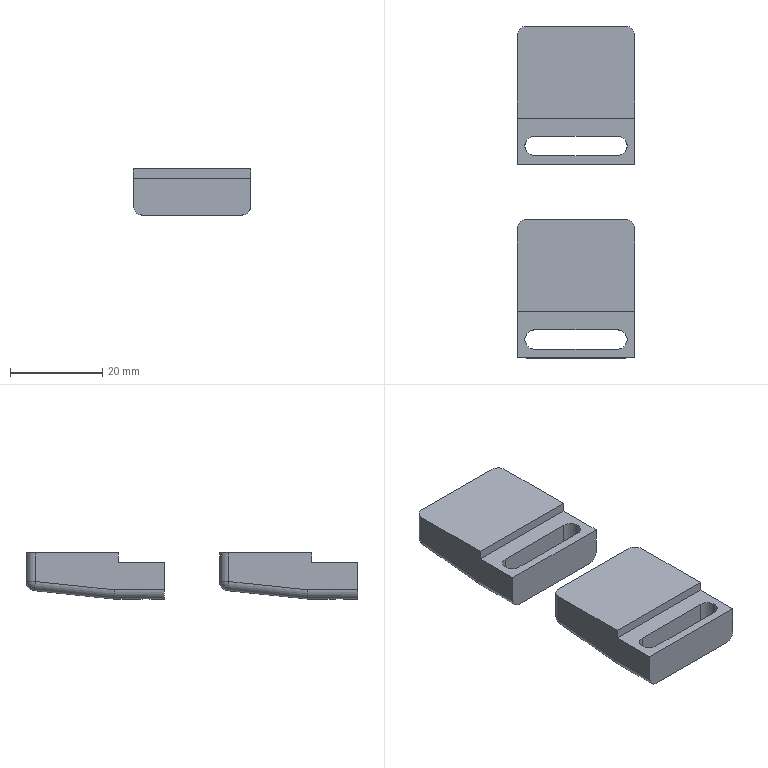NC program | NX | posted with a generic post | part box 25.5 x 72 x 10 mm
Whole program:
N10 G17 G21 G94 G90
(FLOOR_WALL_COPY , TOOL : D80)
N12 T19 M6
N14 G54
N16 G17 G0 G90 X83. Y0. B0. C0. S6500 M3
N18 G43 Z30. H19
N20 Z3.
N22 G94 G1 Z0. F1500.
N24 X78.
N26 X-78.
N28 X-83.
N30 Z3.
N32 G0 Z30.
N34 M5
(ZLEVEL_PROFILE , TOOL : D10)
N36 T15 M6
N38 G54
N40 G17 G0 G90 X-12.133 Y17.85 B0. C0. S9500 M3
N42 G43 Z30. H15
N44 Z1.5
N46 G94 G1 X-5.446 Z1.15 F1000.
N48 X-4.102 Y17.516 Z1.077
N50 X-2.896 Y16.834 Z1.004
N52 X-1.916 Y15.854 Z0.932
N54 X-1.234 Y14.648 Z0.859
N56 X-0.9 Y13.304 Z0.787
N58 Y-13.304 Z-0.608
N60 X-1.234 Y-14.648 Z-0.681
N62 X-1.916 Y-15.854 Z-0.753
N64 X-2.896 Y-16.834 Z-0.826
N66 X-4.102 Y-17.516 Z-0.898
N68 X-5.446 Y-17.85 Z-0.971
N70 X-6. Z-1.
N72 X-34. F3000.
N74 G2 X-41.1 Y-10.75 R7.1
N76 G1 Y10.75
N78 G2 X-34. Y17.85 R7.1
N80 G1 X-6.
N82 G2 X-0.9 Y12.75 R5.1
N84 G1 Y-12.75
N86 G2 X-6. Y-17.85 R5.1
N88 G1 X-33.871 Z-1.486
N90 X-34.258 Y-17.845 Z-1.493
N92 X-34.644 Y-17.821 Z-1.5
N94 X-35.028 Y-17.775 Z-1.507
N96 X-35.41 Y-17.709 Z-1.514
N98 X-35.787 Y-17.621 Z-1.52
N100 X-36.159 Y-17.514 Z-1.527
N102 X-36.524 Y-17.386 Z-1.534
N104 X-36.882 Y-17.239 Z-1.541
N106 X-37.231 Y-17.072 Z-1.547
N108 X-37.571 Y-16.887 Z-1.554
N110 X-37.9 Y-16.683 Z-1.561
N112 X-38.218 Y-16.462 Z-1.568
N114 X-38.523 Y-16.223 Z-1.574
N116 X-38.814 Y-15.969 Z-1.581
N118 X-39.091 Y-15.699 Z-1.588
N120 X-39.353 Y-15.414 Z-1.595
N122 X-39.6 Y-15.115 Z-1.601
N124 X-39.829 Y-14.804 Z-1.608
N126 X-40.041 Y-14.48 Z-1.615
N128 X-40.236 Y-14.145 Z-1.622
N130 X-40.411 Y-13.8 Z-1.628
N132 X-40.568 Y-13.446 Z-1.635
N134 X-40.705 Y-13.084 Z-1.642
N136 X-40.822 Y-12.716 Z-1.649
N138 X-40.919 Y-12.341 Z-1.655
N140 X-40.996 Y-11.961 Z-1.662
N142 X-41.052 Y-11.578 Z-1.669
N144 X-41.086 Y-11.193 Z-1.676
N146 X-41.1 Y-10.806 Z-1.682
N148 Y-10.419 Z-1.689
N150 Y7.387 Z-2.
N152 Y10.75
N154 G2 X-34. Y17.85 R7.1
N156 G1 X-6.
N158 G2 X-0.9 Y12.75 R5.1
N160 G1 Y-12.75
N162 G2 X-6. Y-17.85 R5.1
N164 G1 X-33.871 Z-2.486
N166 X-34.258 Y-17.845 Z-2.493
N168 X-34.644 Y-17.821 Z-2.5
N170 X-35.028 Y-17.775 Z-2.507
N172 X-35.41 Y-17.709 Z-2.514
N174 X-35.787 Y-17.621 Z-2.52
N176 X-36.159 Y-17.514 Z-2.527
N178 X-36.524 Y-17.386 Z-2.534
N180 X-36.882 Y-17.239 Z-2.541
N182 X-37.231 Y-17.072 Z-2.547
N184 X-37.571 Y-16.887 Z-2.554
N186 X-37.9 Y-16.683 Z-2.561
N188 X-38.218 Y-16.462 Z-2.568
N190 X-38.523 Y-16.223 Z-2.574
N192 X-38.814 Y-15.969 Z-2.581
N194 X-39.091 Y-15.699 Z-2.588
N196 X-39.353 Y-15.414 Z-2.595
N198 X-39.6 Y-15.115 Z-2.601
N200 X-39.829 Y-14.804 Z-2.608
N202 X-40.041 Y-14.48 Z-2.615
N204 X-40.236 Y-14.145 Z-2.622
N206 X-40.411 Y-13.8 Z-2.628
N208 X-40.568 Y-13.446 Z-2.635
N210 X-40.705 Y-13.084 Z-2.642
N212 X-40.822 Y-12.716 Z-2.649
N214 X-40.919 Y-12.341 Z-2.655
N216 X-40.996 Y-11.961 Z-2.662
N218 X-41.052 Y-11.578 Z-2.669
N220 X-41.086 Y-11.193 Z-2.676
N222 X-41.1 Y-10.806 Z-2.682
N224 Y-10.419 Z-2.689
N226 Y7.387 Z-3.
N228 Y10.75
N230 G2 X-34. Y17.85 R7.1
N232 G1 X-6.
N234 G2 X-0.9 Y12.75 R5.1
N236 G1 Y-12.75
N238 G2 X-6. Y-17.85 R5.1
N240 G1 X-33.871 Z-3.486
N242 X-34.258 Y-17.845 Z-3.493
N244 X-34.644 Y-17.821 Z-3.5
N246 X-35.028 Y-17.775 Z-3.507
N248 X-35.41 Y-17.709 Z-3.514
N250 X-35.787 Y-17.621 Z-3.52
N252 X-36.159 Y-17.514 Z-3.527
N254 X-36.524 Y-17.386 Z-3.534
N256 X-36.882 Y-17.239 Z-3.541
N258 X-37.231 Y-17.072 Z-3.547
N260 X-37.571 Y-16.887 Z-3.554
N262 X-37.9 Y-16.683 Z-3.561
N264 X-38.218 Y-16.462 Z-3.568
N266 X-38.523 Y-16.223 Z-3.574
N268 X-38.814 Y-15.969 Z-3.581
N270 X-39.091 Y-15.699 Z-3.588
N272 X-39.353 Y-15.414 Z-3.595
N274 X-39.6 Y-15.115 Z-3.601
N276 X-39.829 Y-14.804 Z-3.608
N278 X-40.041 Y-14.48 Z-3.615
N280 X-40.236 Y-14.145 Z-3.622
N282 X-40.411 Y-13.8 Z-3.628
N284 X-40.568 Y-13.446 Z-3.635
N286 X-40.705 Y-13.084 Z-3.642
N288 X-40.822 Y-12.716 Z-3.649
N290 X-40.919 Y-12.341 Z-3.655
N292 X-40.996 Y-11.961 Z-3.662
N294 X-41.052 Y-11.578 Z-3.669
N296 X-41.086 Y-11.193 Z-3.676
N298 X-41.1 Y-10.806 Z-3.682
N300 Y-10.419 Z-3.689
N302 Y7.387 Z-4.
N304 Y10.75
N306 G2 X-34. Y17.85 R7.1
N308 G1 X-6.
N310 G2 X-0.9 Y12.75 R5.1
N312 G1 Y-12.75
N314 G2 X-6. Y-17.85 R5.1
N316 G1 X-33.871 Z-4.486
N318 X-34.258 Y-17.845 Z-4.493
N320 X-34.644 Y-17.821 Z-4.5
N322 X-35.028 Y-17.775 Z-4.507
N324 X-35.41 Y-17.709 Z-4.514
N326 X-35.787 Y-17.621 Z-4.52
N328 X-36.159 Y-17.514 Z-4.527
N330 X-36.524 Y-17.386 Z-4.534
N332 X-36.882 Y-17.239 Z-4.541
N334 X-37.231 Y-17.072 Z-4.547
N336 X-37.571 Y-16.887 Z-4.554
N338 X-37.9 Y-16.683 Z-4.561
N340 X-38.218 Y-16.462 Z-4.568
N342 X-38.523 Y-16.223 Z-4.574
N344 X-38.814 Y-15.969 Z-4.581
N346 X-39.091 Y-15.699 Z-4.588
N348 X-39.353 Y-15.414 Z-4.595
N350 X-39.6 Y-15.115 Z-4.601
N352 X-39.829 Y-14.804 Z-4.608
N354 X-40.041 Y-14.48 Z-4.615
N356 X-40.236 Y-14.145 Z-4.622
N358 X-40.411 Y-13.8 Z-4.628
N360 X-40.568 Y-13.446 Z-4.635
N362 X-40.705 Y-13.084 Z-4.642
N364 X-40.822 Y-12.716 Z-4.649
N366 X-40.919 Y-12.341 Z-4.655
N368 X-40.996 Y-11.961 Z-4.662
N370 X-41.052 Y-11.578 Z-4.669
N372 X-41.086 Y-11.193 Z-4.676
N374 X-41.1 Y-10.806 Z-4.682
N376 Y-10.419 Z-4.689
N378 Y7.387 Z-5.
N380 Y10.75
N382 G2 X-34. Y17.85 R7.1
N384 G1 X-6.
N386 G2 X-0.9 Y12.75 R5.1
N388 G1 Y-12.75
N390 G2 X-6. Y-17.85 R5.1
N392 G1 X-33.871 Z-5.486
N394 X-34.258 Y-17.845 Z-5.493
N396 X-34.644 Y-17.821 Z-5.5
N398 X-35.028 Y-17.775 Z-5.507
N400 X-35.41 Y-17.709 Z-5.514
N402 X-35.787 Y-17.621 Z-5.52
N404 X-36.159 Y-17.514 Z-5.527
N406 X-36.524 Y-17.386 Z-5.534
N408 X-36.882 Y-17.239 Z-5.541
N410 X-37.231 Y-17.072 Z-5.547
N412 X-37.571 Y-16.887 Z-5.554
N414 X-37.9 Y-16.683 Z-5.561
N416 X-38.218 Y-16.462 Z-5.568
N418 X-38.523 Y-16.223 Z-5.574
N420 X-38.814 Y-15.969 Z-5.581
N422 X-39.091 Y-15.699 Z-5.588
N424 X-39.353 Y-15.414 Z-5.595
N426 X-39.6 Y-15.115 Z-5.601
N428 X-39.829 Y-14.804 Z-5.608
N430 X-40.041 Y-14.48 Z-5.615
N432 X-40.236 Y-14.145 Z-5.622
N434 X-40.411 Y-13.8 Z-5.628
N436 X-40.568 Y-13.446 Z-5.635
N438 X-40.705 Y-13.084 Z-5.642
N440 X-40.822 Y-12.716 Z-5.649
N442 X-40.919 Y-12.341 Z-5.655
N444 X-40.996 Y-11.961 Z-5.662
N446 X-41.052 Y-11.578 Z-5.669
N448 X-41.086 Y-11.193 Z-5.676
N450 X-41.1 Y-10.806 Z-5.682
N452 Y-10.419 Z-5.689
N454 Y7.387 Z-6.
N456 Y10.75
N458 G2 X-34. Y17.85 R7.1
N460 G1 X-6.
N462 G2 X-0.9 Y12.75 R5.1
N464 G1 Y-12.75
N466 G2 X-6. Y-17.85 R5.1
N468 G1 X-33.871 Z-6.486
N470 X-34.258 Y-17.845 Z-6.493
N472 X-34.644 Y-17.821 Z-6.5
N474 X-35.028 Y-17.775 Z-6.507
N476 X-35.41 Y-17.709 Z-6.514
N478 X-35.787 Y-17.621 Z-6.52
N480 X-36.159 Y-17.514 Z-6.527
N482 X-36.524 Y-17.386 Z-6.534
N484 X-36.882 Y-17.239 Z-6.541
N486 X-37.231 Y-17.072 Z-6.547
N488 X-37.571 Y-16.887 Z-6.554
N490 X-37.9 Y-16.683 Z-6.561
N492 X-38.218 Y-16.462 Z-6.568
N494 X-38.523 Y-16.223 Z-6.574
N496 X-38.814 Y-15.969 Z-6.581
N498 X-39.091 Y-15.699 Z-6.588
N500 X-39.353 Y-15.414 Z-6.595
N502 X-39.6 Y-15.115 Z-6.601
N504 X-39.829 Y-14.804 Z-6.608
N506 X-40.041 Y-14.48 Z-6.615
N508 X-40.236 Y-14.145 Z-6.622
N510 X-40.411 Y-13.8 Z-6.628
N512 X-40.568 Y-13.446 Z-6.635
N514 X-40.705 Y-13.084 Z-6.642
N516 X-40.822 Y-12.716 Z-6.649
N518 X-40.919 Y-12.341 Z-6.655
N520 X-40.996 Y-11.961 Z-6.662
N522 X-41.052 Y-11.578 Z-6.669
N524 X-41.086 Y-11.193 Z-6.676
N526 X-41.1 Y-10.806 Z-6.682
N528 Y-10.419 Z-6.689
N530 Y7.387 Z-7.
N532 Y10.75
N534 G2 X-34. Y17.85 R7.1
N536 G1 X-6.
N538 G2 X-0.9 Y12.75 R5.1
N540 G1 Y-12.75
N542 G2 X-6. Y-17.85 R5.1
N544 G1 X-33.871 Z-7.486
N546 X-34.258 Y-17.845 Z-7.493
N548 X-34.644 Y-17.821 Z-7.5
N550 X-35.028 Y-17.775 Z-7.507
N552 X-35.41 Y-17.709 Z-7.514
N554 X-35.787 Y-17.621 Z-7.52
N556 X-36.159 Y-17.514 Z-7.527
N558 X-36.524 Y-17.386 Z-7.534
N560 X-36.882 Y-17.239 Z-7.541
N562 X-37.231 Y-17.072 Z-7.547
N564 X-37.571 Y-16.887 Z-7.554
N566 X-37.9 Y-16.683 Z-7.561
N568 X-38.218 Y-16.462 Z-7.568
N570 X-38.523 Y-16.223 Z-7.574
N572 X-38.814 Y-15.969 Z-7.581
N574 X-39.091 Y-15.699 Z-7.588
N576 X-39.353 Y-15.414 Z-7.595
N578 X-39.6 Y-15.115 Z-7.601
N580 X-39.829 Y-14.804 Z-7.608
N582 X-40.041 Y-14.48 Z-7.615
N584 X-40.236 Y-14.145 Z-7.622
N586 X-40.411 Y-13.8 Z-7.628
N588 X-40.568 Y-13.446 Z-7.635
N590 X-40.705 Y-13.084 Z-7.642
N592 X-40.822 Y-12.716 Z-7.649
N594 X-40.919 Y-12.341 Z-7.655
N596 X-40.996 Y-11.961 Z-7.662
N598 X-41.052 Y-11.578 Z-7.669
N600 X-41.086 Y-11.193 Z-7.676
N602 X-41.1 Y-10.806 Z-7.682
N604 Y-10.419 Z-7.689
N606 Y7.387 Z-8.
N608 Y10.75
N610 G2 X-34. Y17.85 R7.1
N612 G1 X-6.
N614 G2 X-0.9 Y12.75 R5.1
N616 G1 Y-12.75
N618 G2 X-6. Y-17.85 R5.1
N620 G1 X-33.871 Z-8.486
N622 X-34.258 Y-17.845 Z-8.493
N624 X-34.644 Y-17.821 Z-8.5
N626 X-35.028 Y-17.775 Z-8.507
N628 X-35.41 Y-17.709 Z-8.514
N630 X-35.787 Y-17.621 Z-8.52
N632 X-36.159 Y-17.514 Z-8.527
N634 X-36.524 Y-17.386 Z-8.534
N636 X-36.882 Y-17.239 Z-8.541
N638 X-37.231 Y-17.072 Z-8.547
N640 X-37.571 Y-16.887 Z-8.554
N642 X-37.9 Y-16.683 Z-8.561
N644 X-38.218 Y-16.462 Z-8.568
N646 X-38.523 Y-16.223 Z-8.574
N648 X-38.814 Y-15.969 Z-8.581
N650 X-39.091 Y-15.699 Z-8.588
N652 X-39.353 Y-15.414 Z-8.595
N654 X-39.6 Y-15.115 Z-8.601
N656 X-39.829 Y-14.804 Z-8.608
N658 X-40.041 Y-14.48 Z-8.615
N660 X-40.236 Y-14.145 Z-8.622
N662 X-40.411 Y-13.8 Z-8.628
N664 X-40.568 Y-13.446 Z-8.635
N666 X-40.705 Y-13.084 Z-8.642
N668 X-40.822 Y-12.716 Z-8.649
N670 X-40.919 Y-12.341 Z-8.655
N672 X-40.996 Y-11.961 Z-8.662
N674 X-41.052 Y-11.578 Z-8.669
N676 X-41.086 Y-11.193 Z-8.676
N678 X-41.1 Y-10.806 Z-8.682
N680 Y-10.419 Z-8.689
N682 Y7.387 Z-9.
N684 Y10.75
N686 G2 X-34. Y17.85 R7.1
N688 G1 X-6.
N690 G2 X-0.9 Y12.75 R5.1
N692 G1 Y-12.75
N694 G2 X-6. Y-17.85 R5.1
N696 G1 X-33.871 Z-9.486
N698 X-34.258 Y-17.845 Z-9.493
N700 X-34.644 Y-17.821 Z-9.5
N702 X-35.028 Y-17.775 Z-9.507
N704 X-35.41 Y-17.709 Z-9.514
N706 X-35.787 Y-17.621 Z-9.52
N708 X-36.159 Y-17.514 Z-9.527
N710 X-36.524 Y-17.386 Z-9.534
N712 X-36.882 Y-17.239 Z-9.541
N714 X-37.231 Y-17.072 Z-9.547
N716 X-37.571 Y-16.887 Z-9.554
N718 X-37.9 Y-16.683 Z-9.561
N720 X-38.218 Y-16.462 Z-9.568
N722 X-38.523 Y-16.223 Z-9.574
N724 X-38.814 Y-15.969 Z-9.581
N726 X-39.091 Y-15.699 Z-9.588
N728 X-39.353 Y-15.414 Z-9.595
N730 X-39.6 Y-15.115 Z-9.601
N732 X-39.829 Y-14.804 Z-9.608
N734 X-40.041 Y-14.48 Z-9.615
N736 X-40.236 Y-14.145 Z-9.622
N738 X-40.411 Y-13.8 Z-9.628
N740 X-40.568 Y-13.446 Z-9.635
N742 X-40.705 Y-13.084 Z-9.642
N744 X-40.822 Y-12.716 Z-9.649
N746 X-40.919 Y-12.341 Z-9.655
N748 X-40.996 Y-11.961 Z-9.662
N750 X-41.052 Y-11.578 Z-9.669
N752 X-41.086 Y-11.193 Z-9.676
N754 X-41.1 Y-10.806 Z-9.682
N756 Y-10.419 Z-9.689
N758 Y7.387 Z-10.
N760 Y10.75
N762 G2 X-34. Y17.85 R7.1
N764 G1 X-6.
N766 G2 X-0.9 Y12.75 R5.1
N768 G1 Y-12.75
N770 G2 X-6. Y-17.85 R5.1
N772 G1 X-34.
N774 G2 X-41.1 Y-10.75 R7.1
N776 G1 Y7.387
N778 Z-8.5
N780 G0 Z53.
N782 X29.867 Y17.85
N784 Z1.5
N786 G1 X36.554 Z1.15 F1000.
N788 X37.898 Y17.516 Z1.077
N790 X39.104 Y16.834 Z1.004
N792 X40.084 Y15.854 Z0.932
N794 X40.766 Y14.648 Z0.859
N796 X41.1 Y13.304 Z0.787
N798 Y-13.304 Z-0.608
N800 X40.766 Y-14.648 Z-0.681
N802 X40.084 Y-15.854 Z-0.753
N804 X39.104 Y-16.834 Z-0.826
N806 X37.898 Y-17.516 Z-0.898
N808 X36.554 Y-17.85 Z-0.971
N810 X36. Z-1.
N812 X8. F3000.
N814 G2 X0.9 Y-10.75 R7.1
N816 G1 Y10.75
N818 G2 X8. Y17.85 R7.1
N820 G1 X36.
N822 G2 X41.1 Y12.75 R5.1
N824 G1 Y-12.75
N826 G2 X36. Y-17.85 R5.1
N828 G1 X8.129 Z-1.486
N830 X7.742 Y-17.845 Z-1.493
N832 X7.356 Y-17.821 Z-1.5
N834 X6.972 Y-17.775 Z-1.507
N836 X6.59 Y-17.709 Z-1.514
N838 X6.213 Y-17.621 Z-1.52
N840 X5.841 Y-17.514 Z-1.527
N842 X5.476 Y-17.386 Z-1.534
N844 X5.118 Y-17.239 Z-1.541
N846 X4.769 Y-17.072 Z-1.547
N848 X4.429 Y-16.887 Z-1.554
N850 X4.1 Y-16.683 Z-1.561
N852 X3.782 Y-16.462 Z-1.568
N854 X3.477 Y-16.223 Z-1.574
N856 X3.186 Y-15.969 Z-1.581
N858 X2.909 Y-15.699 Z-1.588
N860 X2.647 Y-15.414 Z-1.595
N862 X2.4 Y-15.115 Z-1.601
N864 X2.171 Y-14.804 Z-1.608
N866 X1.959 Y-14.48 Z-1.615
N868 X1.764 Y-14.145 Z-1.622
N870 X1.589 Y-13.8 Z-1.628
N872 X1.432 Y-13.446 Z-1.635
N874 X1.295 Y-13.084 Z-1.642
N876 X1.178 Y-12.716 Z-1.649
N878 X1.081 Y-12.341 Z-1.655
N880 X1.004 Y-11.961 Z-1.662
N882 X0.948 Y-11.578 Z-1.669
N884 X0.914 Y-11.193 Z-1.676
N886 X0.9 Y-10.806 Z-1.682
N888 Y-10.419 Z-1.689
N890 Y7.387 Z-2.
N892 Y10.75
N894 G2 X8. Y17.85 R7.1
N896 G1 X36.
N898 G2 X41.1 Y12.75 R5.1
N900 G1 Y-12.75
N902 G2 X36. Y-17.85 R5.1
N904 G1 X8.129 Z-2.486
N906 X7.742 Y-17.845 Z-2.493
N908 X7.356 Y-17.821 Z-2.5
N910 X6.972 Y-17.775 Z-2.507
N912 X6.59 Y-17.709 Z-2.514
N914 X6.213 Y-17.621 Z-2.52
N916 X5.841 Y-17.514 Z-2.527
N918 X5.476 Y-17.386 Z-2.534
N920 X5.118 Y-17.239 Z-2.541
N922 X4.769 Y-17.072 Z-2.547
N924 X4.429 Y-16.887 Z-2.554
N926 X4.1 Y-16.683 Z-2.561
N928 X3.782 Y-16.462 Z-2.568
N930 X3.477 Y-16.223 Z-2.574
N932 X3.186 Y-15.969 Z-2.581
N934 X2.909 Y-15.699 Z-2.588
N936 X2.647 Y-15.414 Z-2.595
N938 X2.4 Y-15.115 Z-2.601
N940 X2.171 Y-14.804 Z-2.608
N942 X1.959 Y-14.48 Z-2.615
N944 X1.764 Y-14.145 Z-2.622
N946 X1.589 Y-13.8 Z-2.628
N948 X1.432 Y-13.446 Z-2.635
N950 X1.295 Y-13.084 Z-2.642
N952 X1.178 Y-12.716 Z-2.649
N954 X1.081 Y-12.341 Z-2.655
N956 X1.004 Y-11.961 Z-2.662
N958 X0.948 Y-11.578 Z-2.669
N960 X0.914 Y-11.193 Z-2.676
N962 X0.9 Y-10.806 Z-2.682
N964 Y-10.419 Z-2.689
N966 Y7.387 Z-3.
N968 Y10.75
N970 G2 X8. Y17.85 R7.1
N972 G1 X36.
N974 G2 X41.1 Y12.75 R5.1
N976 G1 Y-12.75
N978 G2 X36. Y-17.85 R5.1
N980 G1 X8.129 Z-3.486
N982 X7.742 Y-17.845 Z-3.493
N984 X7.356 Y-17.821 Z-3.5
N986 X6.972 Y-17.775 Z-3.507
N988 X6.59 Y-17.709 Z-3.514
N990 X6.213 Y-17.621 Z-3.52
N992 X5.841 Y-17.514 Z-3.527
N994 X5.476 Y-17.386 Z-3.534
N996 X5.118 Y-17.239 Z-3.541
N998 X4.769 Y-17.072 Z-3.547
N1000 X4.429 Y-16.887 Z-3.554
N1002 X4.1 Y-16.683 Z-3.561
N1004 X3.782 Y-16.462 Z-3.568
N1006 X3.477 Y-16.223 Z-3.574
N1008 X3.186 Y-15.969 Z-3.581
N1010 X2.909 Y-15.699 Z-3.588
N1012 X2.647 Y-15.414 Z-3.595
N1014 X2.4 Y-15.115 Z-3.601
N1016 X2.171 Y-14.804 Z-3.608
N1018 X1.959 Y-14.48 Z-3.615
N1020 X1.764 Y-14.145 Z-3.622
N1022 X1.589 Y-13.8 Z-3.628
N1024 X1.432 Y-13.446 Z-3.635
N1026 X1.295 Y-13.084 Z-3.642
N1028 X1.178 Y-12.716 Z-3.649
N1030 X1.081 Y-12.341 Z-3.655
N1032 X1.004 Y-11.961 Z-3.662
N1034 X0.948 Y-11.578 Z-3.669
N1036 X0.914 Y-11.193 Z-3.676
N1038 X0.9 Y-10.806 Z-3.682
N1040 Y-10.419 Z-3.689
N1042 Y7.387 Z-4.
N1044 Y10.75
N1046 G2 X8. Y17.85 R7.1
N1048 G1 X36.
N1050 G2 X41.1 Y12.75 R5.1
N1052 G1 Y-12.75
N1054 G2 X36. Y-17.85 R5.1
N1056 G1 X8.129 Z-4.486
N1058 X7.742 Y-17.845 Z-4.493
N1060 X7.356 Y-17.821 Z-4.5
N1062 X6.972 Y-17.775 Z-4.507
N1064 X6.59 Y-17.709 Z-4.514
N1066 X6.213 Y-17.621 Z-4.52
N1068 X5.841 Y-17.514 Z-4.527
N1070 X5.476 Y-17.386 Z-4.534
N1072 X5.118 Y-17.239 Z-4.541
N1074 X4.769 Y-17.072 Z-4.547
N1076 X4.429 Y-16.887 Z-4.554
N1078 X4.1 Y-16.683 Z-4.561
N1080 X3.782 Y-16.462 Z-4.568
N1082 X3.477 Y-16.223 Z-4.574
N1084 X3.186 Y-15.969 Z-4.581
N1086 X2.909 Y-15.699 Z-4.588
N1088 X2.647 Y-15.414 Z-4.595
N1090 X2.4 Y-15.115 Z-4.601
N1092 X2.171 Y-14.804 Z-4.608
N1094 X1.959 Y-14.48 Z-4.615
N1096 X1.764 Y-14.145 Z-4.622
N1098 X1.589 Y-13.8 Z-4.628
N1100 X1.432 Y-13.446 Z-4.635
N1102 X1.295 Y-13.084 Z-4.642
N1104 X1.178 Y-12.716 Z-4.649
N1106 X1.081 Y-12.341 Z-4.655
N1108 X1.004 Y-11.961 Z-4.662
N1110 X0.948 Y-11.578 Z-4.669
N1112 X0.914 Y-11.193 Z-4.676
N1114 X0.9 Y-10.806 Z-4.682
N1116 Y-10.419 Z-4.689
N1118 Y7.387 Z-5.
N1120 Y10.75
N1122 G2 X8. Y17.85 R7.1
N1124 G1 X36.
N1126 G2 X41.1 Y12.75 R5.1
N1128 G1 Y-12.75
N1130 G2 X36. Y-17.85 R5.1
N1132 G1 X8.129 Z-5.486
N1134 X7.742 Y-17.845 Z-5.493
N1136 X7.356 Y-17.821 Z-5.5
N1138 X6.972 Y-17.775 Z-5.507
N1140 X6.59 Y-17.709 Z-5.514
N1142 X6.213 Y-17.621 Z-5.52
N1144 X5.841 Y-17.514 Z-5.527
N1146 X5.476 Y-17.386 Z-5.534
N1148 X5.118 Y-17.239 Z-5.541
N1150 X4.769 Y-17.072 Z-5.547
N1152 X4.429 Y-16.887 Z-5.554
N1154 X4.1 Y-16.683 Z-5.561
N1156 X3.782 Y-16.462 Z-5.568
N1158 X3.477 Y-16.223 Z-5.574
N1160 X3.186 Y-15.969 Z-5.581
N1162 X2.909 Y-15.699 Z-5.588
N1164 X2.647 Y-15.414 Z-5.595
N1166 X2.4 Y-15.115 Z-5.601
N1168 X2.171 Y-14.804 Z-5.608
N1170 X1.959 Y-14.48 Z-5.615
N1172 X1.764 Y-14.145 Z-5.622
N1174 X1.589 Y-13.8 Z-5.628
N1176 X1.432 Y-13.446 Z-5.635
N1178 X1.295 Y-13.084 Z-5.642
N1180 X1.178 Y-12.716 Z-5.649
N1182 X1.081 Y-12.341 Z-5.655
N1184 X1.004 Y-11.961 Z-5.662
N1186 X0.948 Y-11.578 Z-5.669
N1188 X0.914 Y-11.193 Z-5.676
N1190 X0.9 Y-10.806 Z-5.682
N1192 Y-10.419 Z-5.689
N1194 Y7.387 Z-6.
N1196 Y10.75
N1198 G2 X8. Y17.85 R7.1
N1200 G1 X36.
N1202 G2 X41.1 Y12.75 R5.1
N1204 G1 Y-12.75
N1206 G2 X36. Y-17.85 R5.1
N1208 G1 X8.129 Z-6.486
N1210 X7.742 Y-17.845 Z-6.493
N1212 X7.356 Y-17.821 Z-6.5
N1214 X6.972 Y-17.775 Z-6.507
N1216 X6.59 Y-17.709 Z-6.514
N1218 X6.213 Y-17.621 Z-6.52
N1220 X5.841 Y-17.514 Z-6.527
N1222 X5.476 Y-17.386 Z-6.534
N1224 X5.118 Y-17.239 Z-6.541
N1226 X4.769 Y-17.072 Z-6.547
N1228 X4.429 Y-16.887 Z-6.554
N1230 X4.1 Y-16.683 Z-6.561
N1232 X3.782 Y-16.462 Z-6.568
N1234 X3.477 Y-16.223 Z-6.574
N1236 X3.186 Y-15.969 Z-6.581
N1238 X2.909 Y-15.699 Z-6.588
N1240 X2.647 Y-15.414 Z-6.595
N1242 X2.4 Y-15.115 Z-6.601
N1244 X2.171 Y-14.804 Z-6.608
N1246 X1.959 Y-14.48 Z-6.615
N1248 X1.764 Y-14.145 Z-6.622
N1250 X1.589 Y-13.8 Z-6.628
N1252 X1.432 Y-13.446 Z-6.635
N1254 X1.295 Y-13.084 Z-6.642
N1256 X1.178 Y-12.716 Z-6.649
N1258 X1.081 Y-12.341 Z-6.655
N1260 X1.004 Y-11.961 Z-6.662
N1262 X0.948 Y-11.578 Z-6.669
N1264 X0.914 Y-11.193 Z-6.676
N1266 X0.9 Y-10.806 Z-6.682
N1268 Y-10.419 Z-6.689
N1270 Y7.387 Z-7.
N1272 Y10.75
N1274 G2 X8. Y17.85 R7.1
N1276 G1 X36.
N1278 G2 X41.1 Y12.75 R5.1
N1280 G1 Y-12.75
N1282 G2 X36. Y-17.85 R5.1
N1284 G1 X8.129 Z-7.486
N1286 X7.742 Y-17.845 Z-7.493
N1288 X7.356 Y-17.821 Z-7.5
N1290 X6.972 Y-17.775 Z-7.507
N1292 X6.59 Y-17.709 Z-7.514
N1294 X6.213 Y-17.621 Z-7.52
N1296 X5.841 Y-17.514 Z-7.527
N1298 X5.476 Y-17.386 Z-7.534
N1300 X5.118 Y-17.239 Z-7.541
N1302 X4.769 Y-17.072 Z-7.547
N1304 X4.429 Y-16.887 Z-7.554
N1306 X4.1 Y-16.683 Z-7.561
N1308 X3.782 Y-16.462 Z-7.568
N1310 X3.477 Y-16.223 Z-7.574
N1312 X3.186 Y-15.969 Z-7.581
N1314 X2.909 Y-15.699 Z-7.588
N1316 X2.647 Y-15.414 Z-7.595
N1318 X2.4 Y-15.115 Z-7.601
N1320 X2.171 Y-14.804 Z-7.608
N1322 X1.959 Y-14.48 Z-7.615
N1324 X1.764 Y-14.145 Z-7.622
N1326 X1.589 Y-13.8 Z-7.628
N1328 X1.432 Y-13.446 Z-7.635
N1330 X1.295 Y-13.084 Z-7.642
N1332 X1.178 Y-12.716 Z-7.649
N1334 X1.081 Y-12.341 Z-7.655
N1336 X1.004 Y-11.961 Z-7.662
N1338 X0.948 Y-11.578 Z-7.669
N1340 X0.914 Y-11.193 Z-7.676
N1342 X0.9 Y-10.806 Z-7.682
N1344 Y-10.419 Z-7.689
N1346 Y7.387 Z-8.
N1348 Y10.75
N1350 G2 X8. Y17.85 R7.1
N1352 G1 X36.
N1354 G2 X41.1 Y12.75 R5.1
N1356 G1 Y-12.75
N1358 G2 X36. Y-17.85 R5.1
N1360 G1 X8.129 Z-8.486
N1362 X7.742 Y-17.845 Z-8.493
N1364 X7.356 Y-17.821 Z-8.5
N1366 X6.972 Y-17.775 Z-8.507
N1368 X6.59 Y-17.709 Z-8.514
N1370 X6.213 Y-17.621 Z-8.52
N1372 X5.841 Y-17.514 Z-8.527
N1374 X5.476 Y-17.386 Z-8.534
N1376 X5.118 Y-17.239 Z-8.541
N1378 X4.769 Y-17.072 Z-8.547
N1380 X4.429 Y-16.887 Z-8.554
N1382 X4.1 Y-16.683 Z-8.561
N1384 X3.782 Y-16.462 Z-8.568
N1386 X3.477 Y-16.223 Z-8.574
N1388 X3.186 Y-15.969 Z-8.581
N1390 X2.909 Y-15.699 Z-8.588
N1392 X2.647 Y-15.414 Z-8.595
N1394 X2.4 Y-15.115 Z-8.601
N1396 X2.171 Y-14.804 Z-8.608
N1398 X1.959 Y-14.48 Z-8.615
N1400 X1.764 Y-14.145 Z-8.622
N1402 X1.589 Y-13.8 Z-8.628
N1404 X1.432 Y-13.446 Z-8.635
N1406 X1.295 Y-13.084 Z-8.642
N1408 X1.178 Y-12.716 Z-8.649
N1410 X1.081 Y-12.341 Z-8.655
N1412 X1.004 Y-11.961 Z-8.662
N1414 X0.948 Y-11.578 Z-8.669
N1416 X0.914 Y-11.193 Z-8.676
N1418 X0.9 Y-10.806 Z-8.682
N1420 Y-10.419 Z-8.689
N1422 Y7.387 Z-9.
N1424 Y10.75
N1426 G2 X8. Y17.85 R7.1
N1428 G1 X36.
N1430 G2 X41.1 Y12.75 R5.1
N1432 G1 Y-12.75
N1434 G2 X36. Y-17.85 R5.1
N1436 G1 X8.129 Z-9.486
N1438 X7.742 Y-17.845 Z-9.493
N1440 X7.356 Y-17.821 Z-9.5
N1442 X6.972 Y-17.775 Z-9.507
N1444 X6.59 Y-17.709 Z-9.514
N1446 X6.213 Y-17.621 Z-9.52
N1448 X5.841 Y-17.514 Z-9.527
N1450 X5.476 Y-17.386 Z-9.534
N1452 X5.118 Y-17.239 Z-9.541
N1454 X4.769 Y-17.072 Z-9.547
N1456 X4.429 Y-16.887 Z-9.554
N1458 X4.1 Y-16.683 Z-9.561
N1460 X3.782 Y-16.462 Z-9.568
N1462 X3.477 Y-16.223 Z-9.574
N1464 X3.186 Y-15.969 Z-9.581
N1466 X2.909 Y-15.699 Z-9.588
N1468 X2.647 Y-15.414 Z-9.595
N1470 X2.4 Y-15.115 Z-9.601
N1472 X2.171 Y-14.804 Z-9.608
N1474 X1.959 Y-14.48 Z-9.615
N1476 X1.764 Y-14.145 Z-9.622
N1478 X1.589 Y-13.8 Z-9.628
N1480 X1.432 Y-13.446 Z-9.635
N1482 X1.295 Y-13.084 Z-9.642
N1484 X1.178 Y-12.716 Z-9.649
N1486 X1.081 Y-12.341 Z-9.655
N1488 X1.004 Y-11.961 Z-9.662
N1490 X0.948 Y-11.578 Z-9.669
N1492 X0.914 Y-11.193 Z-9.676
N1494 X0.9 Y-10.806 Z-9.682
N1496 Y-10.419 Z-9.689
N1498 Y7.387 Z-10.
N1500 Y10.75
N1502 G2 X8. Y17.85 R7.1
N1504 G1 X36.
N1506 G2 X41.1 Y12.75 R5.1
N1508 G1 Y-12.75
N1510 G2 X36. Y-17.85 R5.1
N1512 G1 X8.
N1514 G2 X0.9 Y-10.75 R7.1
N1516 G1 Y7.387
N1518 Z-8.5
N1520 G0 Z30.
(FLOOR_WALL , TOOL : D10)
N1522 X-7.393 Y19.25
N1524 Z0.05
N1526 G1 Z-0.95 F1000.
N1528 X-6.816 Y18.25
N1530 G3 X-5.95 Y17.75 R1.
N1532 G1 X-1. F2500.
N1534 Y-17.75
N1536 X-10.9
N1538 Y17.75
N1540 X-5.95
N1542 Y13.25
N1544 X-5.5
N1546 Y-13.25
N1548 X-6.4
N1550 Y13.25
N1552 X-5.95
N1554 G3 X-5.084 Y13.75 R1.
N1556 G1 Z0.05
N1558 G0 X-7.393 Y19.25 Z-0.9
N1560 G1 Z-1.9 F1000.
N1562 X-6.816 Y18.25
N1564 G3 X-5.95 Y17.75 R1.
N1566 G1 X-1. F2500.
N1568 Y-17.75
N1570 X-10.9
N1572 Y17.75
N1574 X-5.95
N1576 Y13.25
N1578 X-5.5
N1580 Y-13.25
N1582 X-6.4
N1584 Y13.25
N1586 X-5.95
N1588 G3 X-5.084 Y13.75 R1.
N1590 G1 Z-0.9
N1592 G0 Z30.
N1594 X42.5 Y1.443
N1596 Z0.05
N1598 G1 Z-0.95 F1000.
N1600 X41.5 Y0.866
N1602 G3 X41. Y0. R1.
N1604 G1 Y-17.75 F2500.
N1606 X31.1
N1608 Y17.75
N1610 X41.
N1612 Y0.
N1614 X36.5
N1616 Y-13.25
N1618 X35.6
N1620 Y13.25
N1622 X36.5
N1624 Y0.
N1626 G3 X37. Y-0.866 R1.
N1628 G1 Z0.05
N1630 G0 X42.5 Y1.443 Z-0.9
N1632 G1 Z-1.9 F1000.
N1634 X41.5 Y0.866
N1636 G3 X41. Y0. R1.
N1638 G1 Y-17.75 F2500.
N1640 X31.1
N1642 Y17.75
N1644 X41.
N1646 Y0.
N1648 X36.5
N1650 Y-13.25
N1652 X35.6
N1654 Y13.25
N1656 X36.5
N1658 Y0.
N1660 G3 X37. Y-0.866 R1.
N1662 G1 Z-0.9
N1664 G0 Z30.
N1666 M5
(ZLEVEL_PROFILE_COPY_1_COPY_COPY_1 , TOOL : D10JING)
N1668 T14 M6
N1670 G54
N1672 G17 G0 G90 X-4.378 Y-19.559 B0. C0. S9500 M3
N1674 G43 Z30. H14
N1676 Z-9.
N1678 G94 G1 Z-10. F1000.
N1680 X-5.134 Y-18.25
N1682 G3 X-6. Y-17.75 R1.
N1684 G1 X-34. F1200.
N1686 G2 X-41. Y-10.75 R7.
N1688 G1 Y10.75
N1690 G2 X-34. Y17.75 R7.
N1692 G1 X-6.
N1694 G2 X-1. Y12.75 R5.
N1696 G1 Y-12.75
N1698 G2 X-6. Y-17.75 R5.
N1700 G3 X-6.866 Y-18.25 R1.
N1702 G1 X-7.732 Y-19.75
N1704 Z-9.
N1706 G0 Z30.
N1708 X37.622 Y-19.559
N1710 Z-9.
N1712 G1 Z-10. F1000.
N1714 X36.866 Y-18.25
N1716 G3 X36. Y-17.75 R1.
N1718 G1 X8. F1200.
N1720 G2 X1. Y-10.75 R7.
N1722 G1 Y10.75
N1724 G2 X8. Y17.75 R7.
N1726 G1 X36.
N1728 G2 X41. Y12.75 R5.
N1730 G1 Y-12.75
N1732 G2 X36. Y-17.75 R5.
N1734 G3 X35.134 Y-18.25 R1.
N1736 G1 X34.268 Y-19.75
N1738 Z-9.
N1740 G0 Z30.
(FLOOR_WALL_1 , TOOL : D10JING)
N1742 X-5.5 Y-5.971
N1744 Z-0.4
N1746 G1 Y0. Z-2. F1250.
N1748 Y13.25
N1750 X-6.
N1752 Y-13.25
N1754 X-5.5
N1756 Y0.
N1758 X-1.
N1760 Y17.75
N1762 X-10.5
N1764 Y-17.75
N1766 X-1.
N1768 Y0.
N1770 G2 X-0.5 Y0.866 R1.
N1772 G1 Z-0.5
N1774 G0 Z30.
N1776 X-9.402 Y19.25
N1778 Z-0.5
N1780 G1 Z-2.
N1782 X-10.5 Y18.616
N1784 G3 X-11. Y17.75 R1.
N1786 G1 Y-17.75
N1788 G3 X-10.5 Y-18.616 R1.
N1790 G1 X-9.402 Y-19.25
N1792 Z-0.5
N1794 G0 Z30.
N1796 X36.5 Y-5.971
N1798 Z-0.4
N1800 G1 Y0. Z-2.
N1802 Y13.25
N1804 X36.
N1806 Y-13.25
N1808 X36.5
N1810 Y0.
N1812 X41.
N1814 Y17.75
N1816 X31.5
N1818 Y-17.75
N1820 X41.
N1822 Y0.
N1824 G2 X41.5 Y0.866 R1.
N1826 G1 X42.5 Y1.443
N1828 Z-0.5
N1830 G0 Z30.
N1832 X32.598 Y19.25
N1834 Z-0.5
N1836 G1 Z-2.
N1838 X31.5 Y18.616
N1840 G3 X31. Y17.75 R1.
N1842 G1 Y-17.75
N1844 G3 X31.5 Y-18.616 R1.
N1846 G1 X32.598 Y-19.25
N1848 Z-0.5
N1850 G0 Z30.
N1852 M5
(ZLEVEL_PROFILE_COPY , TOOL : D3)
N1854 T17 M6
N1856 G54
N1858 G17 G0 G90 X-9.4 Y-3.382 B0. C0. S9500 M3
N1860 G43 Z30. H17
N1862 Z-0.5
N1864 G94 G1 Y9.192 Z-1.159 F1000.
N1866 X-9.644 Y9.52 Z-1.18
N1868 X-10.038 Y9.629 Z-1.202
N1870 X-10.396 Y9.49 Z-1.222
N1872 X-10.6 Y9.192 Z-1.241
N1874 Y-9.192 Z-2.204
N1876 X-10.396 Y-9.49 Z-2.223
N1878 X-10.038 Y-9.629 Z-2.243
N1880 X-9.644 Y-9.52 Z-2.265
N1882 X-9.4 Y-9.192 Z-2.286
N1884 Y-9. Z-2.296
N1886 Y9. F1200.
N1888 G3 X-10. Y9.6 R0.6
N1890 X-10.6 Y9. R0.6
N1892 G1 Y-9.
N1894 G3 X-10. Y-9.6 R0.6
N1896 X-9.4 Y-9. R0.6
N1898 G1 Y7.975 Z-2.593
N1900 Y9.
N1902 G3 X-10. Y9.6 R0.6
N1904 X-10.6 Y9. R0.6
N1906 G1 Y-9.
N1908 G3 X-10. Y-9.6 R0.6
N1910 X-9.4 Y-9. R0.6
N1912 G1 Y7.975 Z-2.889
N1914 Y9.
N1916 G3 X-10. Y9.6 R0.6
N1918 X-10.6 Y9. R0.6
N1920 G1 Y-9.
N1922 G3 X-10. Y-9.6 R0.6
N1924 X-9.4 Y-9. R0.6
N1926 G1 Y7.975 Z-3.185
N1928 Y9.
N1930 G3 X-10. Y9.6 R0.6
N1932 X-10.6 Y9. R0.6
N1934 G1 Y-9.
N1936 G3 X-10. Y-9.6 R0.6
N1938 X-9.4 Y-9. R0.6
N1940 G1 Y7.975 Z-3.481
N1942 Y9.
N1944 G3 X-10. Y9.6 R0.6
N1946 X-10.6 Y9. R0.6
N1948 G1 Y-9.
N1950 G3 X-10. Y-9.6 R0.6
N1952 X-9.4 Y-9. R0.6
N1954 G1 Y7.975 Z-3.778
N1956 Y9.
N1958 G3 X-10. Y9.6 R0.6
N1960 X-10.6 Y9. R0.6
N1962 G1 Y-9.
N1964 G3 X-10. Y-9.6 R0.6
N1966 X-9.4 Y-9. R0.6
N1968 G1 Y7.975 Z-4.074
N1970 Y9.
N1972 G3 X-10. Y9.6 R0.6
N1974 X-10.6 Y9. R0.6
N1976 G1 Y-9.
N1978 G3 X-10. Y-9.6 R0.6
N1980 X-9.4 Y-9. R0.6
N1982 G1 Y7.975 Z-4.37
N1984 Y9.
N1986 G3 X-10. Y9.6 R0.6
N1988 X-10.6 Y9. R0.6
N1990 G1 Y-9.
N1992 G3 X-10. Y-9.6 R0.6
N1994 X-9.4 Y-9. R0.6
N1996 G1 Y7.975 Z-4.667
N1998 Y9.
N2000 G3 X-10. Y9.6 R0.6
N2002 X-10.6 Y9. R0.6
N2004 G1 Y-9.
N2006 G3 X-10. Y-9.6 R0.6
N2008 X-9.4 Y-9. R0.6
N2010 G1 Y7.975 Z-4.963
N2012 Y9.
N2014 G3 X-10. Y9.6 R0.6
N2016 X-10.6 Y9. R0.6
N2018 G1 Y-9.
N2020 G3 X-10. Y-9.6 R0.6
N2022 X-9.4 Y-9. R0.6
N2024 G1 Y7.975 Z-5.259
N2026 Y9.
N2028 G3 X-10. Y9.6 R0.6
N2030 X-10.6 Y9. R0.6
N2032 G1 Y-9.
N2034 G3 X-10. Y-9.6 R0.6
N2036 X-9.4 Y-9. R0.6
N2038 G1 Y7.975 Z-5.556
N2040 Y9.
N2042 G3 X-10. Y9.6 R0.6
N2044 X-10.6 Y9. R0.6
N2046 G1 Y-9.
N2048 G3 X-10. Y-9.6 R0.6
N2050 X-9.4 Y-9. R0.6
N2052 G1 Y7.975 Z-5.852
N2054 Y9.
N2056 G3 X-10. Y9.6 R0.6
N2058 X-10.6 Y9. R0.6
N2060 G1 Y-9.
N2062 G3 X-10. Y-9.6 R0.6
N2064 X-9.4 Y-9. R0.6
N2066 G1 Y7.975 Z-6.148
N2068 Y9.
N2070 G3 X-10. Y9.6 R0.6
N2072 X-10.6 Y9. R0.6
N2074 G1 Y-9.
N2076 G3 X-10. Y-9.6 R0.6
N2078 X-9.4 Y-9. R0.6
N2080 G1 Y7.975 Z-6.444
N2082 Y9.
N2084 G3 X-10. Y9.6 R0.6
N2086 X-10.6 Y9. R0.6
N2088 G1 Y-9.
N2090 G3 X-10. Y-9.6 R0.6
N2092 X-9.4 Y-9. R0.6
N2094 G1 Y7.975 Z-6.741
N2096 Y9.
N2098 G3 X-10. Y9.6 R0.6
N2100 X-10.6 Y9. R0.6
N2102 G1 Y-9.
N2104 G3 X-10. Y-9.6 R0.6
N2106 X-9.4 Y-9. R0.6
N2108 G1 Y7.975 Z-7.037
N2110 Y9.
N2112 G3 X-10. Y9.6 R0.6
N2114 X-10.6 Y9. R0.6
N2116 G1 Y-9.
N2118 G3 X-10. Y-9.6 R0.6
N2120 X-9.4 Y-9. R0.6
N2122 G1 Y7.975 Z-7.333
N2124 Y9.
N2126 G3 X-10. Y9.6 R0.6
N2128 X-10.6 Y9. R0.6
N2130 G1 Y-9.
N2132 G3 X-10. Y-9.6 R0.6
N2134 X-9.4 Y-9. R0.6
N2136 G1 Y7.975 Z-7.63
N2138 Y9.
N2140 G3 X-10. Y9.6 R0.6
N2142 X-10.6 Y9. R0.6
N2144 G1 Y-9.
N2146 G3 X-10. Y-9.6 R0.6
N2148 X-9.4 Y-9. R0.6
N2150 G1 Y7.975 Z-7.926
N2152 Y9.
N2154 G3 X-10. Y9.6 R0.6
N2156 X-10.6 Y9. R0.6
N2158 G1 Y-9.
N2160 G3 X-10. Y-9.6 R0.6
N2162 X-9.4 Y-9. R0.6
N2164 G1 Y7.975 Z-8.222
N2166 Y9.
N2168 G3 X-10. Y9.6 R0.6
N2170 X-10.6 Y9. R0.6
N2172 G1 Y-9.
N2174 G3 X-10. Y-9.6 R0.6
N2176 X-9.4 Y-9. R0.6
N2178 G1 Y7.975 Z-8.519
N2180 Y9.
N2182 G3 X-10. Y9.6 R0.6
N2184 X-10.6 Y9. R0.6
N2186 G1 Y-9.
N2188 G3 X-10. Y-9.6 R0.6
N2190 X-9.4 Y-9. R0.6
N2192 G1 Y7.975 Z-8.815
N2194 Y9.
N2196 G3 X-10. Y9.6 R0.6
N2198 X-10.6 Y9. R0.6
N2200 G1 Y-9.
N2202 G3 X-10. Y-9.6 R0.6
N2204 X-9.4 Y-9. R0.6
N2206 G1 Y7.975 Z-9.111
N2208 Y9.
N2210 G3 X-10. Y9.6 R0.6
N2212 X-10.6 Y9. R0.6
N2214 G1 Y-9.
N2216 G3 X-10. Y-9.6 R0.6
N2218 X-9.4 Y-9. R0.6
N2220 G1 Y7.975 Z-9.407
N2222 Y9.
N2224 G3 X-10. Y9.6 R0.6
N2226 X-10.6 Y9. R0.6
N2228 G1 Y-9.
N2230 G3 X-10. Y-9.6 R0.6
N2232 X-9.4 Y-9. R0.6
N2234 G1 Y7.975 Z-9.704
N2236 Y9.
N2238 G3 X-10. Y9.6 R0.6
N2240 X-10.6 Y9. R0.6
N2242 G1 Y-9.
N2244 G3 X-10. Y-9.6 R0.6
N2246 X-9.4 Y-9. R0.6
N2248 G1 Y7.975 Z-10.
N2250 Y9.
N2252 G3 X-10. Y9.6 R0.6
N2254 X-10.6 Y9. R0.6
N2256 G1 Y-9.
N2258 G3 X-10. Y-9.6 R0.6
N2260 X-9.4 Y-9. R0.6
N2262 G1 Y7.975
N2264 Z-8.5
N2266 G0 Z30.
N2268 X32.6 Y-3.382
N2270 Z-0.5
N2272 G1 Y9.192 Z-1.159 F1000.
N2274 X32.356 Y9.52 Z-1.18
N2276 X31.962 Y9.629 Z-1.202
N2278 X31.604 Y9.49 Z-1.222
N2280 X31.4 Y9.192 Z-1.241
N2282 Y-9.192 Z-2.204
N2284 X31.604 Y-9.49 Z-2.223
N2286 X31.962 Y-9.629 Z-2.243
N2288 X32.356 Y-9.52 Z-2.265
N2290 X32.6 Y-9.192 Z-2.286
N2292 Y-9. Z-2.296
N2294 Y9. F1200.
N2296 G3 X32. Y9.6 R0.6
N2298 X31.4 Y9. R0.6
N2300 G1 Y-9.
N2302 G3 X32. Y-9.6 R0.6
N2304 X32.6 Y-9. R0.6
N2306 G1 Y7.975 Z-2.593
N2308 Y9.
N2310 G3 X32. Y9.6 R0.6
N2312 X31.4 Y9. R0.6
N2314 G1 Y-9.
N2316 G3 X32. Y-9.6 R0.6
N2318 X32.6 Y-9. R0.6
N2320 G1 Y7.975 Z-2.889
N2322 Y9.
N2324 G3 X32. Y9.6 R0.6
N2326 X31.4 Y9. R0.6
N2328 G1 Y-9.
N2330 G3 X32. Y-9.6 R0.6
N2332 X32.6 Y-9. R0.6
N2334 G1 Y7.975 Z-3.185
N2336 Y9.
N2338 G3 X32. Y9.6 R0.6
N2340 X31.4 Y9. R0.6
N2342 G1 Y-9.
N2344 G3 X32. Y-9.6 R0.6
N2346 X32.6 Y-9. R0.6
N2348 G1 Y7.975 Z-3.481
N2350 Y9.
N2352 G3 X32. Y9.6 R0.6
N2354 X31.4 Y9. R0.6
N2356 G1 Y-9.
N2358 G3 X32. Y-9.6 R0.6
N2360 X32.6 Y-9. R0.6
N2362 G1 Y7.975 Z-3.778
N2364 Y9.
N2366 G3 X32. Y9.6 R0.6
N2368 X31.4 Y9. R0.6
N2370 G1 Y-9.
N2372 G3 X32. Y-9.6 R0.6
N2374 X32.6 Y-9. R0.6
N2376 G1 Y7.975 Z-4.074
N2378 Y9.
N2380 G3 X32. Y9.6 R0.6
N2382 X31.4 Y9. R0.6
N2384 G1 Y-9.
N2386 G3 X32. Y-9.6 R0.6
N2388 X32.6 Y-9. R0.6
N2390 G1 Y7.975 Z-4.37
N2392 Y9.
N2394 G3 X32. Y9.6 R0.6
N2396 X31.4 Y9. R0.6
N2398 G1 Y-9.
N2400 G3 X32. Y-9.6 R0.6
N2402 X32.6 Y-9. R0.6
N2404 G1 Y7.975 Z-4.667
N2406 Y9.
N2408 G3 X32. Y9.6 R0.6
N2410 X31.4 Y9. R0.6
N2412 G1 Y-9.
N2414 G3 X32. Y-9.6 R0.6
N2416 X32.6 Y-9. R0.6
N2418 G1 Y7.975 Z-4.963
N2420 Y9.
N2422 G3 X32. Y9.6 R0.6
N2424 X31.4 Y9. R0.6
N2426 G1 Y-9.
N2428 G3 X32. Y-9.6 R0.6
N2430 X32.6 Y-9. R0.6
N2432 G1 Y7.975 Z-5.259
N2434 Y9.
N2436 G3 X32. Y9.6 R0.6
N2438 X31.4 Y9. R0.6
N2440 G1 Y-9.
N2442 G3 X32. Y-9.6 R0.6
N2444 X32.6 Y-9. R0.6
N2446 G1 Y7.975 Z-5.556
N2448 Y9.
N2450 G3 X32. Y9.6 R0.6
N2452 X31.4 Y9. R0.6
N2454 G1 Y-9.
N2456 G3 X32. Y-9.6 R0.6
N2458 X32.6 Y-9. R0.6
N2460 G1 Y7.975 Z-5.852
N2462 Y9.
N2464 G3 X32. Y9.6 R0.6
N2466 X31.4 Y9. R0.6
N2468 G1 Y-9.
N2470 G3 X32. Y-9.6 R0.6
N2472 X32.6 Y-9. R0.6
N2474 G1 Y7.975 Z-6.148
N2476 Y9.
N2478 G3 X32. Y9.6 R0.6
N2480 X31.4 Y9. R0.6
N2482 G1 Y-9.
N2484 G3 X32. Y-9.6 R0.6
N2486 X32.6 Y-9. R0.6
N2488 G1 Y7.975 Z-6.444
N2490 Y9.
N2492 G3 X32. Y9.6 R0.6
N2494 X31.4 Y9. R0.6
N2496 G1 Y-9.
N2498 G3 X32. Y-9.6 R0.6
N2500 X32.6 Y-9. R0.6
N2502 G1 Y7.975 Z-6.741
N2504 Y9.
N2506 G3 X32. Y9.6 R0.6
N2508 X31.4 Y9. R0.6
N2510 G1 Y-9.
N2512 G3 X32. Y-9.6 R0.6
N2514 X32.6 Y-9. R0.6
N2516 G1 Y7.975 Z-7.037
N2518 Y9.
N2520 G3 X32. Y9.6 R0.6
N2522 X31.4 Y9. R0.6
N2524 G1 Y-9.
N2526 G3 X32. Y-9.6 R0.6
N2528 X32.6 Y-9. R0.6
N2530 G1 Y7.975 Z-7.333
N2532 Y9.
N2534 G3 X32. Y9.6 R0.6
N2536 X31.4 Y9. R0.6
N2538 G1 Y-9.
N2540 G3 X32. Y-9.6 R0.6
N2542 X32.6 Y-9. R0.6
N2544 G1 Y7.975 Z-7.63
N2546 Y9.
N2548 G3 X32. Y9.6 R0.6
N2550 X31.4 Y9. R0.6
N2552 G1 Y-9.
N2554 G3 X32. Y-9.6 R0.6
N2556 X32.6 Y-9. R0.6
N2558 G1 Y7.975 Z-7.926
N2560 Y9.
N2562 G3 X32. Y9.6 R0.6
N2564 X31.4 Y9. R0.6
N2566 G1 Y-9.
N2568 G3 X32. Y-9.6 R0.6
N2570 X32.6 Y-9. R0.6
N2572 G1 Y7.975 Z-8.222
N2574 Y9.
N2576 G3 X32. Y9.6 R0.6
N2578 X31.4 Y9. R0.6
N2580 G1 Y-9.
N2582 G3 X32. Y-9.6 R0.6
N2584 X32.6 Y-9. R0.6
N2586 G1 Y7.975 Z-8.519
N2588 Y9.
N2590 G3 X32. Y9.6 R0.6
N2592 X31.4 Y9. R0.6
N2594 G1 Y-9.
N2596 G3 X32. Y-9.6 R0.6
N2598 X32.6 Y-9. R0.6
N2600 G1 Y7.975 Z-8.815
N2602 Y9.
N2604 G3 X32. Y9.6 R0.6
N2606 X31.4 Y9. R0.6
N2608 G1 Y-9.
N2610 G3 X32. Y-9.6 R0.6
N2612 X32.6 Y-9. R0.6
N2614 G1 Y7.975 Z-9.111
N2616 Y9.
N2618 G3 X32. Y9.6 R0.6
N2620 X31.4 Y9. R0.6
N2622 G1 Y-9.
N2624 G3 X32. Y-9.6 R0.6
N2626 X32.6 Y-9. R0.6
N2628 G1 Y7.975 Z-9.407
N2630 Y9.
N2632 G3 X32. Y9.6 R0.6
N2634 X31.4 Y9. R0.6
N2636 G1 Y-9.
N2638 G3 X32. Y-9.6 R0.6
N2640 X32.6 Y-9. R0.6
N2642 G1 Y7.975 Z-9.704
N2644 Y9.
N2646 G3 X32. Y9.6 R0.6
N2648 X31.4 Y9. R0.6
N2650 G1 Y-9.
N2652 G3 X32. Y-9.6 R0.6
N2654 X32.6 Y-9. R0.6
N2656 G1 Y7.975 Z-10.
N2658 Y9.
N2660 G3 X32. Y9.6 R0.6
N2662 X31.4 Y9. R0.6
N2664 G1 Y-9.
N2666 G3 X32. Y-9.6 R0.6
N2668 X32.6 Y-9. R0.6
N2670 G1 Y7.975
N2672 Z-8.5
N2674 G0 Z30.
N2676 M5
(PLANAR_MILL_COPY_COPY_COPY_COPY_COPY_COPY_1_COPY_1 , TOOL : D6A45)
N2678 T01 M6
N2680 G54
N2682 G17 G0 G90 X-37.4 Y-0.866 B0. C0. S9500 M3
N2684 G43 Z30. H1
N2686 Z0.5
N2688 G94 G1 Z-1. F1250.
N2690 G3 X-36.9 Y0. R1.
N2692 G1 Y10.75
N2694 G2 X-34. Y13.65 R2.9
N2696 G1 X-16.
N2698 G2 X-15.1 Y12.75 R0.9
N2700 G1 Y-12.75
N2702 G2 X-16. Y-13.65 R0.9
N2704 G1 X-34.
N2706 G2 X-36.9 Y-10.75 R2.9
N2708 G1 Y0.
N2710 G3 X-37.4 Y0.866 R1.
N2712 G1 Z0.5
N2714 G0 Z30.
N2716 X27.4
N2718 Z0.5
N2720 G1 Z-1.
N2722 G3 X26.9 Y0. R1.
N2724 G1 Y-12.75
N2726 G2 X26. Y-13.65 R0.9
N2728 G1 X8.
N2730 G2 X5.1 Y-10.75 R2.9
N2732 G1 Y10.75
N2734 G2 X8. Y13.65 R2.9
N2736 G1 X26.
N2738 G2 X26.9 Y12.75 R0.9
N2740 G1 Y0.
N2742 G3 X27.4 Y-0.866 R1.
N2744 G1 Z0.5
N2746 G0 Z30.
(PLANAR_MILL_COPY_COPY_COPY_COPY_COPY_COPY_1_COPY_1_COPY , TOOL : D6A45)
N2748 X-10. Y1.27
N2750 Z-1.5
N2752 G1 Z-3.
N2754 X-10.7 Y0.866
N2756 G3 X-11.2 Y0. R1.
N2758 G1 Y-9.
N2760 G3 X-10. Y-10.2 R1.2
N2762 X-8.8 Y-9. R1.2
N2764 G1 Y9.
N2766 G3 X-10. Y10.2 R1.2
N2768 X-11.2 Y9. R1.2
N2770 G1 Y0.
N2772 G3 X-10.7 Y-0.866 R1.
N2774 G1 X-10. Y-1.27
N2776 Z-1.5
N2778 G0 Z30.
N2780 X-11.908 Y15.063
N2782 Z-1.5
N2784 G1 Z-3.
N2786 X-12.357 Y14.615
N2788 G3 X-12.618 Y13.65 R1.
N2790 G1 X-6.1
N2792 G2 X-5.1 Y12.65 R1.
N2794 G1 Y-12.65
N2796 G2 X-6.1 Y-13.65 R1.
N2798 G1 X-12.618
N2800 G3 X-12.357 Y-14.615 R1.
N2802 G1 X-11.908 Y-15.063
N2804 Z-1.5
N2806 G0 Z30.
N2808 X30.092 Y15.063
N2810 Z-1.5
N2812 G1 Z-3.
N2814 X29.643 Y14.615
N2816 G3 X29.382 Y13.65 R1.
N2818 G1 X35.9
N2820 G2 X36.9 Y12.65 R1.
N2822 G1 Y-12.65
N2824 G2 X35.9 Y-13.65 R1.
N2826 G1 X29.382
N2828 G3 X29.643 Y-14.615 R1.
N2830 G1 X30.092 Y-15.063
N2832 Z-1.5
N2834 G0 Z30.
N2836 X32. Y-1.27
N2838 Z-1.5
N2840 G1 Z-3.
N2842 X32.7 Y-0.866
N2844 G3 X33.2 Y0. R1.
N2846 G1 Y9.
N2848 G3 X32. Y10.2 R1.2
N2850 X30.8 Y9. R1.2
N2852 G1 Y-9.
N2854 G3 X32. Y-10.2 R1.2
N2856 X33.2 Y-9. R1.2
N2858 G1 Y0.
N2860 G3 X32.7 Y0.866 R1.
N2862 G1 X32. Y1.27
N2864 Z-1.5
N2866 G0 Z30.
N2868 M5
N2870 M2